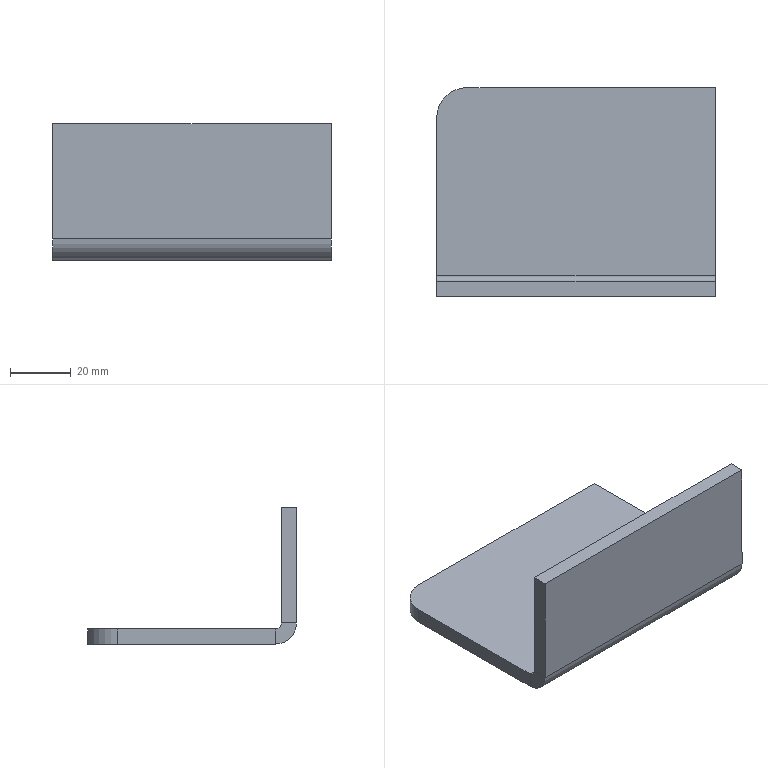Part | SolidWorks | features Fillet 1, FlatPattern 1, SM3dBend 1, SMBaseFlange 1, SheetMetal 1 | 1 solid | 15 faces | box 92 x 68.996 x 44.996 mm | volume 49140 mm3 | plane 12 | cylinder 3 | commonest cylinder face diameters 4 x1 14 x1 20 x1
STEP:
#1=CARTESIAN_POINT('',(46.,-15.466,39.996));
#2=VERTEX_POINT('',#1);
#3=CARTESIAN_POINT('',(46.,-15.466,2.));
#4=VERTEX_POINT('',#3);
#5=CARTESIAN_POINT('',(46.,-15.466,-67.064));
#6=DIRECTION('',(0.,0.,-1.));
#7=VECTOR('',#6,1000.);
#8=LINE('',#5,#7);
#9=EDGE_CURVE('',#2,#4,#8,.T.);
#10=ORIENTED_EDGE('',*,*,#9,.T.);
#11=CARTESIAN_POINT('',(46.,-10.466,2.));
#12=VERTEX_POINT('',#11);
#13=CARTESIAN_POINT('',(46.,-15.466,2.));
#14=DIRECTION('',(0.,1.,0.));
#15=VECTOR('',#14,1000.);
#16=LINE('',#13,#15);
#17=EDGE_CURVE('',#4,#12,#16,.T.);
#18=ORIENTED_EDGE('',*,*,#17,.T.);
#19=CARTESIAN_POINT('',(46.,-10.466,39.996));
#20=VERTEX_POINT('',#19);
#21=CARTESIAN_POINT('',(46.,-10.466,-67.064));
#22=DIRECTION('',(0.,0.,-1.));
#23=VECTOR('',#22,1000.);
#24=LINE('',#21,#23);
#25=EDGE_CURVE('',#20,#12,#24,.T.);
#26=ORIENTED_EDGE('',*,*,#25,.F.);
#27=CARTESIAN_POINT('',(46.,-15.466,39.996));
#28=DIRECTION('',(0.,1.,0.));
#29=VECTOR('',#28,1000.);
#30=LINE('',#27,#29);
#31=EDGE_CURVE('',#2,#20,#30,.T.);
#32=ORIENTED_EDGE('',*,*,#31,.F.);
#33=EDGE_LOOP('',(#10,#18,#26,#32));
#34=FACE_OUTER_BOUND('',#33,.T.);
#35=CARTESIAN_POINT('',(46.,-15.466,-67.064));
#36=DIRECTION('',(1.,0.,0.));
#37=DIRECTION('',(0.,0.,-1.));
#38=AXIS2_PLACEMENT_3D('',#35,#36,#37);
#39=PLANE('',#38);
#40=ADVANCED_FACE('',(#34),#39,.T.);
#41=CARTESIAN_POINT('',(-46.,-10.466,2.));
#42=VERTEX_POINT('',#41);
#43=CARTESIAN_POINT('',(-46.,-10.466,39.996));
#44=VERTEX_POINT('',#43);
#45=CARTESIAN_POINT('',(-46.,-10.466,-67.064));
#46=DIRECTION('',(0.,0.,1.));
#47=VECTOR('',#46,1000.);
#48=LINE('',#45,#47);
#49=EDGE_CURVE('',#42,#44,#48,.T.);
#50=ORIENTED_EDGE('',*,*,#49,.F.);
#51=CARTESIAN_POINT('',(-46.,-15.466,2.));
#52=VERTEX_POINT('',#51);
#53=CARTESIAN_POINT('',(-46.,-15.466,2.));
#54=DIRECTION('',(0.,-1.,0.));
#55=VECTOR('',#54,1000.);
#56=LINE('',#53,#55);
#57=EDGE_CURVE('',#42,#52,#56,.T.);
#58=ORIENTED_EDGE('',*,*,#57,.T.);
#59=CARTESIAN_POINT('',(-46.,-15.466,39.996));
#60=VERTEX_POINT('',#59);
#61=CARTESIAN_POINT('',(-46.,-15.466,-67.064));
#62=DIRECTION('',(0.,0.,1.));
#63=VECTOR('',#62,1000.);
#64=LINE('',#61,#63);
#65=EDGE_CURVE('',#52,#60,#64,.T.);
#66=ORIENTED_EDGE('',*,*,#65,.T.);
#67=CARTESIAN_POINT('',(-46.,-15.466,39.996));
#68=DIRECTION('',(0.,1.,0.));
#69=VECTOR('',#68,1000.);
#70=LINE('',#67,#69);
#71=EDGE_CURVE('',#60,#44,#70,.T.);
#72=ORIENTED_EDGE('',*,*,#71,.T.);
#73=EDGE_LOOP('',(#50,#58,#66,#72));
#74=FACE_OUTER_BOUND('',#73,.T.);
#75=CARTESIAN_POINT('',(-46.,-15.466,-67.064));
#76=DIRECTION('',(-1.,0.,0.));
#77=DIRECTION('',(0.,0.,1.));
#78=AXIS2_PLACEMENT_3D('',#75,#76,#77);
#79=PLANE('',#78);
#80=ADVANCED_FACE('',(#74),#79,.T.);
#81=ORIENTED_EDGE('',*,*,#25,.T.);
#82=CARTESIAN_POINT('',(0.,-10.466,2.));
#83=DIRECTION('',(-1.,0.,0.));
#84=VECTOR('',#83,1000.);
#85=LINE('',#82,#84);
#86=EDGE_CURVE('',#12,#42,#85,.T.);
#87=ORIENTED_EDGE('',*,*,#86,.T.);
#88=ORIENTED_EDGE('',*,*,#49,.T.);
#89=CARTESIAN_POINT('',(-46.,-10.466,39.996));
#90=DIRECTION('',(1.,0.,0.));
#91=VECTOR('',#90,1000.);
#92=LINE('',#89,#91);
#93=EDGE_CURVE('',#44,#20,#92,.T.);
#94=ORIENTED_EDGE('',*,*,#93,.T.);
#95=EDGE_LOOP('',(#81,#87,#88,#94));
#96=FACE_OUTER_BOUND('',#95,.T.);
#97=CARTESIAN_POINT('',(0.,-10.466,-13.534));
#98=DIRECTION('',(0.,1.,0.));
#99=DIRECTION('',(1.,0.,0.));
#100=AXIS2_PLACEMENT_3D('',#97,#98,#99);
#101=PLANE('',#100);
#102=ADVANCED_FACE('',(#96),#101,.T.);
#103=ORIENTED_EDGE('',*,*,#93,.F.);
#104=ORIENTED_EDGE('',*,*,#71,.F.);
#105=CARTESIAN_POINT('',(-46.,-15.466,39.996));
#106=DIRECTION('',(1.,0.,0.));
#107=VECTOR('',#106,1000.);
#108=LINE('',#105,#107);
#109=EDGE_CURVE('',#60,#2,#108,.T.);
#110=ORIENTED_EDGE('',*,*,#109,.T.);
#111=ORIENTED_EDGE('',*,*,#31,.T.);
#112=EDGE_LOOP('',(#103,#104,#110,#111));
#113=FACE_OUTER_BOUND('',#112,.T.);
#114=CARTESIAN_POINT('',(-46.,-15.466,39.996));
#115=DIRECTION('',(0.,0.,1.));
#116=DIRECTION('',(0.,-1.,0.));
#117=AXIS2_PLACEMENT_3D('',#114,#115,#116);
#118=PLANE('',#117);
#119=ADVANCED_FACE('',(#113),#118,.T.);
#120=CARTESIAN_POINT('',(0.,-15.466,2.));
#121=DIRECTION('',(-1.,0.,0.));
#122=VECTOR('',#121,1000.);
#123=LINE('',#120,#122);
#124=EDGE_CURVE('',#4,#52,#123,.T.);
#125=ORIENTED_EDGE('',*,*,#124,.F.);
#126=ORIENTED_EDGE('',*,*,#9,.F.);
#127=ORIENTED_EDGE('',*,*,#109,.F.);
#128=ORIENTED_EDGE('',*,*,#65,.F.);
#129=EDGE_LOOP('',(#125,#126,#127,#128));
#130=FACE_OUTER_BOUND('',#129,.T.);
#131=CARTESIAN_POINT('',(0.,-15.466,-13.534));
#132=DIRECTION('',(0.,1.,0.));
#133=DIRECTION('',(1.,0.,0.));
#134=AXIS2_PLACEMENT_3D('',#131,#132,#133);
#135=PLANE('',#134);
#136=ADVANCED_FACE('',(#130),#135,.F.);
#137=CARTESIAN_POINT('',(46.,53.53,-5.));
#138=VERTEX_POINT('',#137);
#139=CARTESIAN_POINT('',(-36.,53.53,-5.));
#140=VERTEX_POINT('',#139);
#141=CARTESIAN_POINT('',(-46.,53.53,-5.));
#142=DIRECTION('',(-1.,0.,0.));
#143=VECTOR('',#142,1000.);
#144=LINE('',#141,#143);
#145=EDGE_CURVE('',#138,#140,#144,.T.);
#146=ORIENTED_EDGE('',*,*,#145,.T.);
#147=CARTESIAN_POINT('',(-36.,53.53,0.));
#148=VERTEX_POINT('',#147);
#149=CARTESIAN_POINT('',(-36.,53.53,-5.));
#150=DIRECTION('',(0.,0.,1.));
#151=VECTOR('',#150,1000.);
#152=LINE('',#149,#151);
#153=EDGE_CURVE('',#140,#148,#152,.T.);
#154=ORIENTED_EDGE('',*,*,#153,.T.);
#155=CARTESIAN_POINT('',(46.,53.53,0.));
#156=VERTEX_POINT('',#155);
#157=CARTESIAN_POINT('',(-46.,53.53,0.));
#158=DIRECTION('',(-1.,0.,0.));
#159=VECTOR('',#158,1000.);
#160=LINE('',#157,#159);
#161=EDGE_CURVE('',#156,#148,#160,.T.);
#162=ORIENTED_EDGE('',*,*,#161,.F.);
#163=CARTESIAN_POINT('',(46.,53.53,-5.));
#164=DIRECTION('',(0.,0.,1.));
#165=VECTOR('',#164,1000.);
#166=LINE('',#163,#165);
#167=EDGE_CURVE('',#138,#156,#166,.T.);
#168=ORIENTED_EDGE('',*,*,#167,.F.);
#169=EDGE_LOOP('',(#146,#154,#162,#168));
#170=FACE_OUTER_BOUND('',#169,.T.);
#171=CARTESIAN_POINT('',(-46.,53.53,-5.));
#172=DIRECTION('',(0.,1.,0.));
#173=DIRECTION('',(0.,0.,1.));
#174=AXIS2_PLACEMENT_3D('',#171,#172,#173);
#175=PLANE('',#174);
#176=ADVANCED_FACE('',(#170),#175,.T.);
#177=CARTESIAN_POINT('',(-46.,43.53,-5.));
#178=VERTEX_POINT('',#177);
#179=CARTESIAN_POINT('',(-46.,-8.466,-5.));
#180=VERTEX_POINT('',#179);
#181=CARTESIAN_POINT('',(-46.,53.53,-5.));
#182=DIRECTION('',(0.,-1.,0.));
#183=VECTOR('',#182,1000.);
#184=LINE('',#181,#183);
#185=EDGE_CURVE('',#178,#180,#184,.T.);
#186=ORIENTED_EDGE('',*,*,#185,.F.);
#187=CARTESIAN_POINT('',(-36.,43.53,-5.));
#188=DIRECTION('',(0.,0.,-1.));
#189=DIRECTION('',(1.,0.,0.));
#190=AXIS2_PLACEMENT_3D('',#187,#188,#189);
#191=CIRCLE('',#190,10.);
#192=EDGE_CURVE('',#178,#140,#191,.T.);
#193=ORIENTED_EDGE('',*,*,#192,.T.);
#194=ORIENTED_EDGE('',*,*,#145,.F.);
#195=CARTESIAN_POINT('',(46.,-8.466,-5.));
#196=VERTEX_POINT('',#195);
#197=CARTESIAN_POINT('',(46.,53.53,-5.));
#198=DIRECTION('',(0.,1.,0.));
#199=VECTOR('',#198,1000.);
#200=LINE('',#197,#199);
#201=EDGE_CURVE('',#196,#138,#200,.T.);
#202=ORIENTED_EDGE('',*,*,#201,.F.);
#203=CARTESIAN_POINT('',(0.,-8.466,-5.));
#204=DIRECTION('',(-1.,0.,0.));
#205=VECTOR('',#204,1000.);
#206=LINE('',#203,#205);
#207=EDGE_CURVE('',#196,#180,#206,.T.);
#208=ORIENTED_EDGE('',*,*,#207,.T.);
#209=EDGE_LOOP('',(#186,#193,#194,#202,#208));
#210=FACE_OUTER_BOUND('',#209,.T.);
#211=CARTESIAN_POINT('',(0.,0.,-5.));
#212=DIRECTION('',(0.,0.,1.));
#213=DIRECTION('',(1.,0.,0.));
#214=AXIS2_PLACEMENT_3D('',#211,#212,#213);
#215=PLANE('',#214);
#216=ADVANCED_FACE('',(#210),#215,.F.);
#217=CARTESIAN_POINT('',(-46.,43.53,0.));
#218=VERTEX_POINT('',#217);
#219=CARTESIAN_POINT('',(-46.,-8.466,0.));
#220=VERTEX_POINT('',#219);
#221=CARTESIAN_POINT('',(-46.,53.53,0.));
#222=DIRECTION('',(0.,-1.,0.));
#223=VECTOR('',#222,1000.);
#224=LINE('',#221,#223);
#225=EDGE_CURVE('',#218,#220,#224,.T.);
#226=ORIENTED_EDGE('',*,*,#225,.F.);
#227=CARTESIAN_POINT('',(-46.,43.53,-5.));
#228=DIRECTION('',(0.,0.,-1.));
#229=VECTOR('',#228,1000.);
#230=LINE('',#227,#229);
#231=EDGE_CURVE('',#218,#178,#230,.T.);
#232=ORIENTED_EDGE('',*,*,#231,.T.);
#233=ORIENTED_EDGE('',*,*,#185,.T.);
#234=CARTESIAN_POINT('',(-46.,-8.466,-5.));
#235=DIRECTION('',(0.,0.,-1.));
#236=VECTOR('',#235,1000.);
#237=LINE('',#234,#236);
#238=EDGE_CURVE('',#220,#180,#237,.T.);
#239=ORIENTED_EDGE('',*,*,#238,.F.);
#240=EDGE_LOOP('',(#226,#232,#233,#239));
#241=FACE_OUTER_BOUND('',#240,.T.);
#242=CARTESIAN_POINT('',(-46.,53.53,-5.));
#243=DIRECTION('',(-1.,0.,0.));
#244=DIRECTION('',(0.,-1.,0.));
#245=AXIS2_PLACEMENT_3D('',#242,#243,#244);
#246=PLANE('',#245);
#247=ADVANCED_FACE('',(#241),#246,.T.);
#248=ORIENTED_EDGE('',*,*,#161,.T.);
#249=CARTESIAN_POINT('',(-36.,43.53,0.));
#250=DIRECTION('',(0.,0.,1.));
#251=DIRECTION('',(1.,0.,0.));
#252=AXIS2_PLACEMENT_3D('',#249,#250,#251);
#253=CIRCLE('',#252,10.);
#254=EDGE_CURVE('',#148,#218,#253,.T.);
#255=ORIENTED_EDGE('',*,*,#254,.T.);
#256=ORIENTED_EDGE('',*,*,#225,.T.);
#257=CARTESIAN_POINT('',(46.,-8.466,0.));
#258=VERTEX_POINT('',#257);
#259=CARTESIAN_POINT('',(0.,-8.466,0.));
#260=DIRECTION('',(-1.,0.,0.));
#261=VECTOR('',#260,1000.);
#262=LINE('',#259,#261);
#263=EDGE_CURVE('',#258,#220,#262,.T.);
#264=ORIENTED_EDGE('',*,*,#263,.F.);
#265=CARTESIAN_POINT('',(46.,53.53,0.));
#266=DIRECTION('',(0.,1.,0.));
#267=VECTOR('',#266,1000.);
#268=LINE('',#265,#267);
#269=EDGE_CURVE('',#258,#156,#268,.T.);
#270=ORIENTED_EDGE('',*,*,#269,.T.);
#271=EDGE_LOOP('',(#248,#255,#256,#264,#270));
#272=FACE_OUTER_BOUND('',#271,.T.);
#273=CARTESIAN_POINT('',(0.,0.,0.));
#274=DIRECTION('',(0.,0.,1.));
#275=DIRECTION('',(1.,0.,0.));
#276=AXIS2_PLACEMENT_3D('',#273,#274,#275);
#277=PLANE('',#276);
#278=ADVANCED_FACE('',(#272),#277,.T.);
#279=CARTESIAN_POINT('',(46.,-8.466,-5.));
#280=DIRECTION('',(0.,0.,1.));
#281=VECTOR('',#280,1000.);
#282=LINE('',#279,#281);
#283=EDGE_CURVE('',#196,#258,#282,.T.);
#284=ORIENTED_EDGE('',*,*,#283,.F.);
#285=ORIENTED_EDGE('',*,*,#201,.T.);
#286=ORIENTED_EDGE('',*,*,#167,.T.);
#287=ORIENTED_EDGE('',*,*,#269,.F.);
#288=EDGE_LOOP('',(#284,#285,#286,#287));
#289=FACE_OUTER_BOUND('',#288,.T.);
#290=CARTESIAN_POINT('',(46.,53.53,-5.));
#291=DIRECTION('',(1.,0.,0.));
#292=DIRECTION('',(0.,1.,0.));
#293=AXIS2_PLACEMENT_3D('',#290,#291,#292);
#294=PLANE('',#293);
#295=ADVANCED_FACE('',(#289),#294,.T.);
#296=ORIENTED_EDGE('',*,*,#283,.T.);
#297=CARTESIAN_POINT('',(46.,-8.466,2.));
#298=DIRECTION('',(-1.,0.,0.));
#299=DIRECTION('',(0.,0.,1.));
#300=AXIS2_PLACEMENT_3D('',#297,#298,#299);
#301=CIRCLE('',#300,2.);
#302=EDGE_CURVE('',#258,#12,#301,.T.);
#303=ORIENTED_EDGE('',*,*,#302,.T.);
#304=ORIENTED_EDGE('',*,*,#17,.F.);
#305=CARTESIAN_POINT('',(46.,-8.466,2.));
#306=DIRECTION('',(-1.,0.,0.));
#307=DIRECTION('',(0.,0.,-1.));
#308=AXIS2_PLACEMENT_3D('',#305,#306,#307);
#309=CIRCLE('',#308,7.);
#310=EDGE_CURVE('',#196,#4,#309,.T.);
#311=ORIENTED_EDGE('',*,*,#310,.F.);
#312=EDGE_LOOP('',(#296,#303,#304,#311));
#313=FACE_OUTER_BOUND('',#312,.T.);
#314=CARTESIAN_POINT('',(46.,-8.466,2.));
#315=DIRECTION('',(1.,0.,0.));
#316=DIRECTION('',(0.,0.,-1.));
#317=AXIS2_PLACEMENT_3D('',#314,#315,#316);
#318=PLANE('',#317);
#319=ADVANCED_FACE('',(#313),#318,.T.);
#320=ORIENTED_EDGE('',*,*,#57,.F.);
#321=CARTESIAN_POINT('',(-46.,-8.466,2.));
#322=DIRECTION('',(1.,0.,0.));
#323=DIRECTION('',(0.,0.,1.));
#324=AXIS2_PLACEMENT_3D('',#321,#322,#323);
#325=CIRCLE('',#324,2.);
#326=EDGE_CURVE('',#42,#220,#325,.T.);
#327=ORIENTED_EDGE('',*,*,#326,.T.);
#328=ORIENTED_EDGE('',*,*,#238,.T.);
#329=CARTESIAN_POINT('',(-46.,-8.466,2.));
#330=DIRECTION('',(1.,0.,0.));
#331=DIRECTION('',(0.,0.,1.));
#332=AXIS2_PLACEMENT_3D('',#329,#330,#331);
#333=CIRCLE('',#332,7.);
#334=EDGE_CURVE('',#52,#180,#333,.T.);
#335=ORIENTED_EDGE('',*,*,#334,.F.);
#336=EDGE_LOOP('',(#320,#327,#328,#335));
#337=FACE_OUTER_BOUND('',#336,.T.);
#338=CARTESIAN_POINT('',(-46.,-8.466,2.));
#339=DIRECTION('',(-1.,0.,0.));
#340=DIRECTION('',(0.,0.,1.));
#341=AXIS2_PLACEMENT_3D('',#338,#339,#340);
#342=PLANE('',#341);
#343=ADVANCED_FACE('',(#337),#342,.T.);
#344=ORIENTED_EDGE('',*,*,#334,.T.);
#345=ORIENTED_EDGE('',*,*,#207,.F.);
#346=ORIENTED_EDGE('',*,*,#310,.T.);
#347=ORIENTED_EDGE('',*,*,#124,.T.);
#348=EDGE_LOOP('',(#344,#345,#346,#347));
#349=FACE_OUTER_BOUND('',#348,.T.);
#350=CARTESIAN_POINT('',(92.407,-8.466,2.));
#351=DIRECTION('',(-1.,0.,0.));
#352=DIRECTION('',(0.,0.,1.));
#353=AXIS2_PLACEMENT_3D('',#350,#351,#352);
#354=CYLINDRICAL_SURFACE('',#353,7.);
#355=ADVANCED_FACE('',(#349),#354,.T.);
#356=ORIENTED_EDGE('',*,*,#326,.F.);
#357=ORIENTED_EDGE('',*,*,#86,.F.);
#358=ORIENTED_EDGE('',*,*,#302,.F.);
#359=ORIENTED_EDGE('',*,*,#263,.T.);
#360=EDGE_LOOP('',(#356,#357,#358,#359));
#361=FACE_OUTER_BOUND('',#360,.T.);
#362=CARTESIAN_POINT('',(92.407,-8.466,2.));
#363=DIRECTION('',(-1.,0.,0.));
#364=DIRECTION('',(0.,0.,1.));
#365=AXIS2_PLACEMENT_3D('',#362,#363,#364);
#366=CYLINDRICAL_SURFACE('',#365,2.);
#367=ADVANCED_FACE('',(#361),#366,.F.);
#368=ORIENTED_EDGE('',*,*,#192,.F.);
#369=ORIENTED_EDGE('',*,*,#231,.F.);
#370=ORIENTED_EDGE('',*,*,#254,.F.);
#371=ORIENTED_EDGE('',*,*,#153,.F.);
#372=EDGE_LOOP('',(#368,#369,#370,#371));
#373=FACE_OUTER_BOUND('',#372,.T.);
#374=CARTESIAN_POINT('',(-36.,43.53,-5.));
#375=DIRECTION('',(0.,0.,1.));
#376=DIRECTION('',(1.,0.,0.));
#377=AXIS2_PLACEMENT_3D('',#374,#375,#376);
#378=CYLINDRICAL_SURFACE('',#377,10.);
#379=ADVANCED_FACE('',(#373),#378,.T.);
#380=CLOSED_SHELL('',(#40,#80,#102,#119,#136,#176,#216,#247,#278,#295,#319,#343,#355,#367,#379));
#381=MANIFOLD_SOLID_BREP('',#380);
#382=CARTESIAN_POINT('',(0.,0.,0.));
#383=DIRECTION('',(0.,0.,1.));
#384=DIRECTION('',(1.,0.,0.));
#385=AXIS2_PLACEMENT_3D('',#382,#383,#384);
#386=(LENGTH_UNIT()NAMED_UNIT(*)SI_UNIT(.MILLI.,.METRE.));
#387=UNCERTAINTY_MEASURE_WITH_UNIT(LENGTH_MEASURE(0.00001),#386,'','');
#388=(NAMED_UNIT(*)PLANE_ANGLE_UNIT()SI_UNIT($,.RADIAN.));
#389=(NAMED_UNIT(*)SI_UNIT($,.STERADIAN.)SOLID_ANGLE_UNIT());
#390=(GEOMETRIC_REPRESENTATION_CONTEXT(3)GLOBAL_UNCERTAINTY_ASSIGNED_CONTEXT((#387))GLOBAL_UNIT_ASSIGNED_CONTEXT((#386,#388,#389))REPRESENTATION_CONTEXT('',''));
#391=ADVANCED_BREP_SHAPE_REPRESENTATION('',(#381,#385),#390);